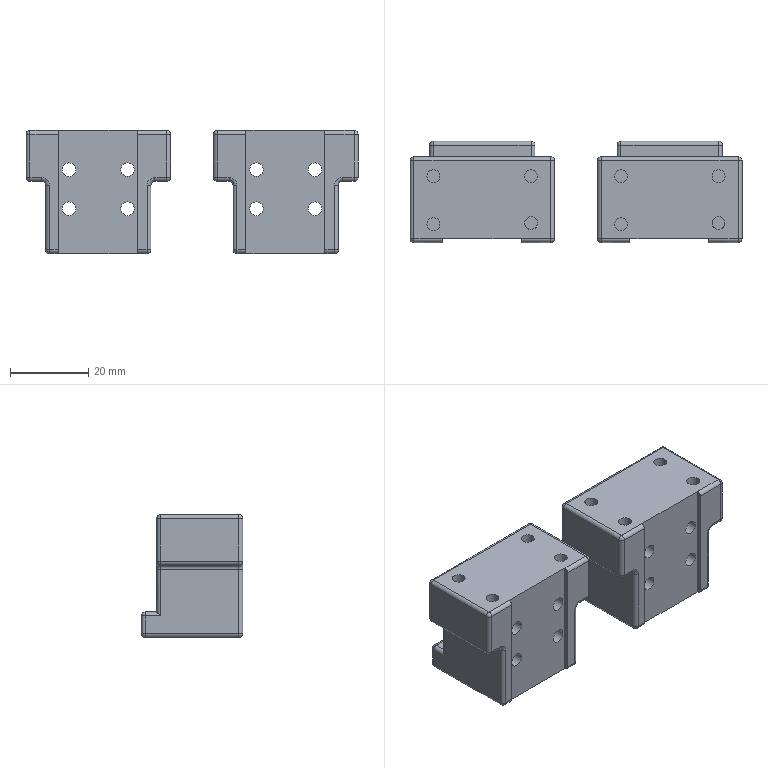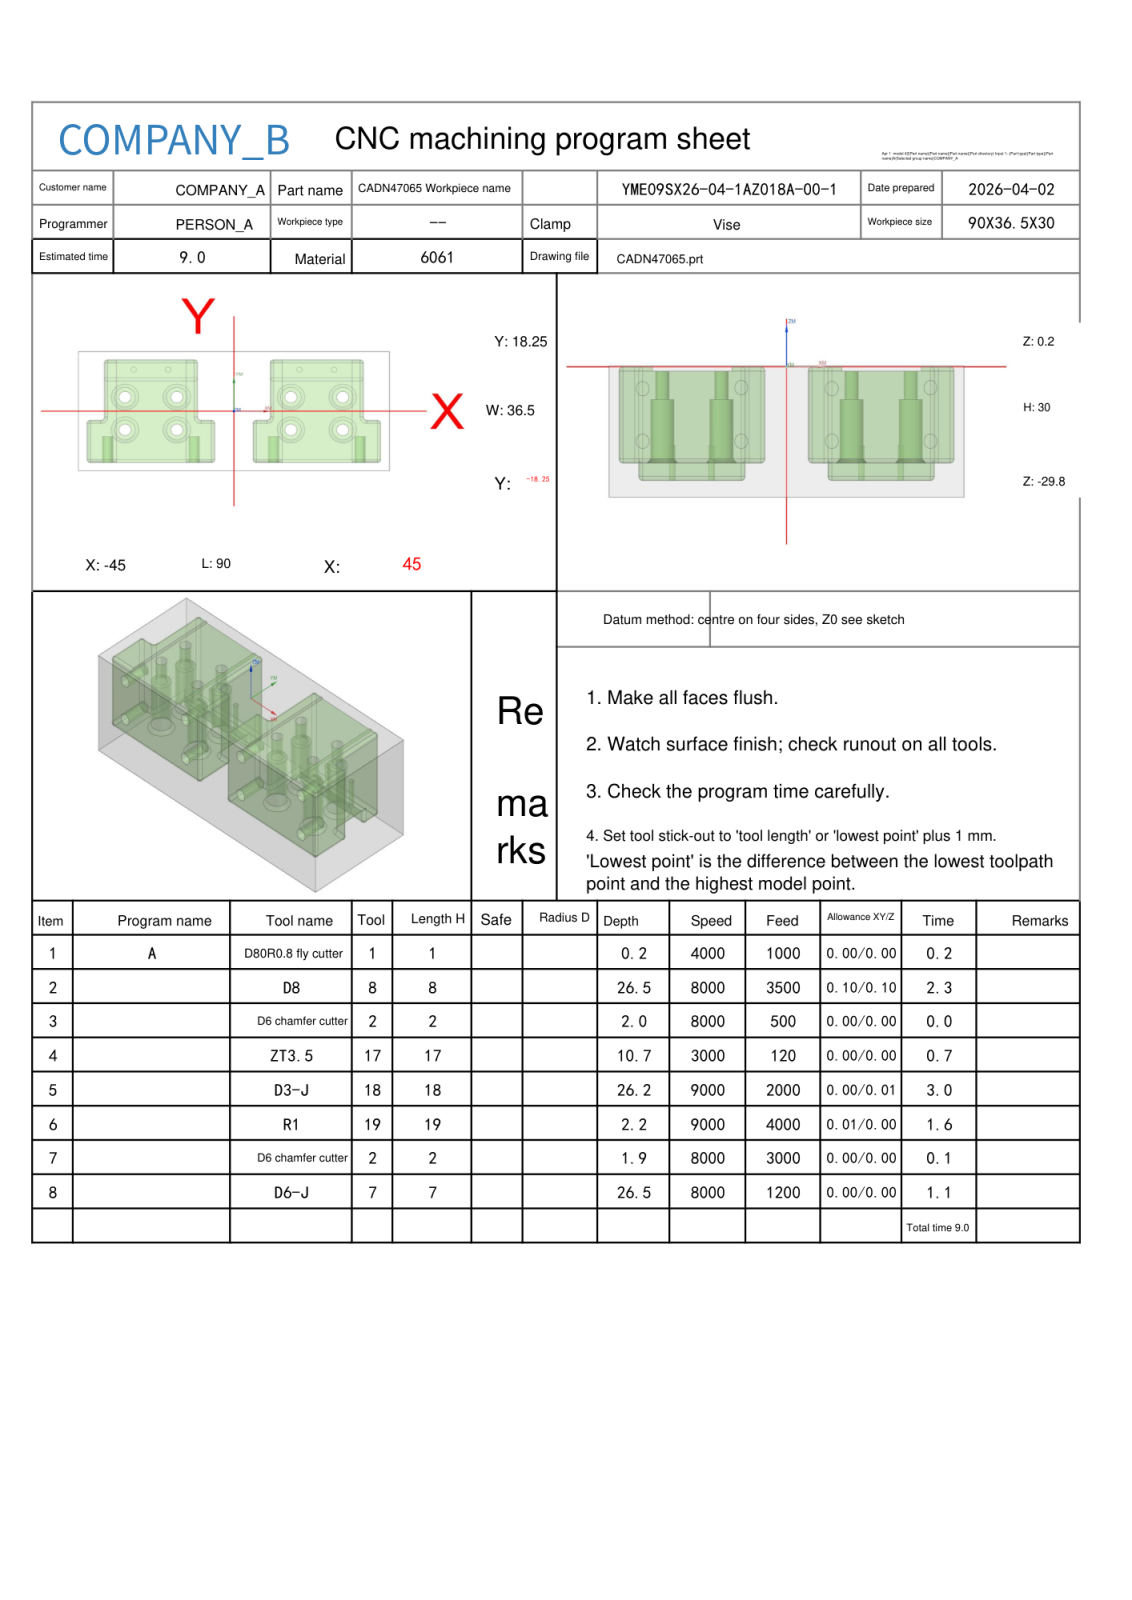NC program | NX | posted by the shop | part box 85 x 26 x 31.5 mm
Lines 3074 to 4231 of 17928:
N5 T18 M06
(D3-J  D=3. R=0. H=18 ce=0.00 di=0.01)
G00 G90 G54 X5.414 Y-.858 M03 S9000
G43 H18 Z20.
M08
Z-.75
G01 X5.417 Y-.864 Z-.818 F1600.
X5.424 Y-.88 Z-.88
X5.435 Y-.905 Z-.935
X5.45 Y-.937 Z-.983
X5.47 Y-.975 Z-1.026
X5.493 Y-1.017 Z-1.064
X5.519 Y-1.062 Z-1.095
X5.549 Y-1.108 Z-1.123
X5.582 Y-1.154 Z-1.145
X5.618 Y-1.198 Z-1.163
X5.656 Y-1.24 Z-1.177
X5.697 Y-1.276 Z-1.187
X5.739 Y-1.306 Z-1.194
X5.784 Y-1.328 Z-1.198
X5.831 Y-1.341 Z-1.2
G02 X6.5 Y-1.25 I.669 J-2.409 F2000.
G01 X9.
Y2.291
X8.985 Y2.32
X8.943 Y2.324 Z-1.202
X8.876 Y2.306 Z-1.205
X8.787 Y2.268 Z-1.208
X8.68 Y2.211 Z-1.213
X8.558 Y2.137 Z-1.218
X8.344 Y1.994 Z-1.228
X8.103 Y1.816 Z-1.239
X7.815 Y1.584 Z-1.254
X7.399 Y1.201 Z-1.276
X7.008 Y.785 Z-1.299
X6.651 Y.343 Z-1.323
X6.335 Y-.117 Z-1.345
X6.152 Y-.428 Z-1.359
X6.016 Y-.686 Z-1.371
X5.91 Y-.911 Z-1.38
X5.858 Y-1.038 Z-1.386
X5.82 Y-1.148 Z-1.39
X5.797 Y-1.236 Z-1.394
X5.79 Y-1.3 Z-1.397
X5.801 Y-1.336 Z-1.399
X5.831 Y-1.341
G02 X6.5 Y-1.25 I.669 J-2.409
G01 X9.
Y2.291
X8.985 Y2.32 Z-1.4
X8.943 Y2.324 Z-1.402
X8.876 Y2.306 Z-1.404
X8.787 Y2.268 Z-1.408
X8.68 Y2.211 Z-1.413
X8.558 Y2.137 Z-1.418
X8.344 Y1.994 Z-1.428
X8.103 Y1.816 Z-1.439
X7.815 Y1.584 Z-1.453
X7.399 Y1.201 Z-1.476
X7.008 Y.785 Z-1.499
X6.651 Y.343 Z-1.522
X6.335 Y-.117 Z-1.545
X6.152 Y-.428 Z-1.559
X6.016 Y-.686 Z-1.57
X5.91 Y-.911 Z-1.58
X5.858 Y-1.038 Z-1.585
X5.82 Y-1.148 Z-1.59
X5.797 Y-1.236 Z-1.594
X5.79 Y-1.3 Z-1.596
X5.801 Y-1.336 Z-1.598
X5.831 Y-1.341 Z-1.599
G02 X6.5 Y-1.25 I.669 J-2.409
G01 X9.
Y2.291
X8.985 Y2.32
X8.943 Y2.324 Z-1.601
X8.876 Y2.306 Z-1.604
X8.787 Y2.268 Z-1.608
X8.68 Y2.211 Z-1.612
X8.558 Y2.137 Z-1.618
X8.344 Y1.994 Z-1.627
X8.103 Y1.816 Z-1.639
X7.815 Y1.584 Z-1.653
X7.399 Y1.201 Z-1.675
X7.008 Y.785 Z-1.699
X6.651 Y.343 Z-1.722
X6.335 Y-.117 Z-1.744
X6.152 Y-.428 Z-1.759
X6.016 Y-.686 Z-1.77
X5.91 Y-.911 Z-1.78
X5.858 Y-1.038 Z-1.785
X5.82 Y-1.148 Z-1.79
X5.797 Y-1.236 Z-1.793
X5.79 Y-1.3 Z-1.796
X5.801 Y-1.336 Z-1.798
X5.831 Y-1.341
G02 X6.5 Y-1.25 I.669 J-2.409
G01 X9.
Y2.291
X8.985 Y2.32 Z-1.799
X8.943 Y2.324 Z-1.801
X8.876 Y2.306 Z-1.804
X8.787 Y2.268 Z-1.807
X8.68 Y2.211 Z-1.812
X8.558 Y2.137 Z-1.817
X8.344 Y1.994 Z-1.827
X8.103 Y1.816 Z-1.838
X7.815 Y1.584 Z-1.852
X7.399 Y1.201 Z-1.875
X7.008 Y.785 Z-1.898
X6.651 Y.343 Z-1.921
X6.335 Y-.117 Z-1.944
X6.152 Y-.428 Z-1.958
X6.016 Y-.686 Z-1.969
X5.91 Y-.911 Z-1.979
X5.858 Y-1.038 Z-1.984
X5.82 Y-1.148 Z-1.989
X5.797 Y-1.236 Z-1.993
X5.79 Y-1.3 Z-1.996
X5.801 Y-1.336 Z-1.997
X5.831 Y-1.341 Z-1.998
G02 X6.5 Y-1.25 I.669 J-2.409
G01 X9.
Y2.291
X8.985 Y2.32 Z-1.999
X8.943 Y2.324 Z-2.
X8.876 Y2.306 Z-2.003
X8.787 Y2.268 Z-2.007
X8.68 Y2.211 Z-2.012
X8.558 Y2.137 Z-2.017
X8.344 Y1.994 Z-2.027
X8.103 Y1.816 Z-2.038
X7.815 Y1.584 Z-2.052
X7.399 Y1.201 Z-2.075
X7.008 Y.785 Z-2.098
X6.651 Y.343 Z-2.121
X6.335 Y-.117 Z-2.144
X6.152 Y-.428 Z-2.158
X6.016 Y-.686 Z-2.169
X5.91 Y-.911 Z-2.179
X5.858 Y-1.038 Z-2.184
X5.82 Y-1.148 Z-2.189
X5.797 Y-1.236 Z-2.192
X5.79 Y-1.3 Z-2.195
X5.801 Y-1.336 Z-2.197
X5.831 Y-1.341 Z-2.198
G02 X6.5 Y-1.25 I.669 J-2.409
G01 X9.
Y2.291
X8.985 Y2.32
X8.943 Y2.324 Z-2.2
X8.876 Y2.306 Z-2.203
X8.787 Y2.268 Z-2.207
X8.68 Y2.211 Z-2.211
X8.558 Y2.137 Z-2.216
X8.344 Y1.994 Z-2.226
X8.103 Y1.816 Z-2.237
X7.815 Y1.584 Z-2.252
X7.399 Y1.201 Z-2.274
X7.008 Y.785 Z-2.297
X6.651 Y.343 Z-2.321
X6.335 Y-.117 Z-2.343
X6.152 Y-.428 Z-2.357
X6.016 Y-.686 Z-2.369
X5.91 Y-.911 Z-2.378
X5.858 Y-1.038 Z-2.384
X5.82 Y-1.148 Z-2.388
X5.797 Y-1.236 Z-2.392
X5.79 Y-1.3 Z-2.395
X5.801 Y-1.336 Z-2.397
X5.831 Y-1.341
G02 X6.5 Y-1.25 I.669 J-2.409
G01 X9.
Y2.291
X8.985 Y2.32 Z-2.398
X8.943 Y2.324 Z-2.4
X8.876 Y2.306 Z-2.402
X8.787 Y2.268 Z-2.406
X8.68 Y2.211 Z-2.411
X8.558 Y2.137 Z-2.416
X8.344 Y1.994 Z-2.426
X8.103 Y1.816 Z-2.437
X7.815 Y1.584 Z-2.451
X7.399 Y1.201 Z-2.474
X7.008 Y.785 Z-2.497
X6.651 Y.343 Z-2.52
X6.335 Y-.117 Z-2.543
X6.152 Y-.428 Z-2.557
X6.016 Y-.686 Z-2.568
X5.91 Y-.911 Z-2.578
X5.858 Y-1.038 Z-2.583
X5.82 Y-1.148 Z-2.588
X5.797 Y-1.236 Z-2.592
X5.79 Y-1.3 Z-2.594
X5.801 Y-1.336 Z-2.596
X5.831 Y-1.341 Z-2.597
G02 X6.5 Y-1.25 I.669 J-2.409
G01 X9.
Y2.291
X8.985 Y2.32
X8.943 Y2.324 Z-2.599
X8.876 Y2.306 Z-2.602
X8.787 Y2.268 Z-2.606
X8.68 Y2.211 Z-2.61
X8.558 Y2.137 Z-2.616
X8.344 Y1.994 Z-2.625
X8.103 Y1.816 Z-2.637
X7.815 Y1.584 Z-2.651
X7.399 Y1.201 Z-2.673
X7.008 Y.785 Z-2.697
X6.651 Y.343 Z-2.72
X6.335 Y-.117 Z-2.742
X6.152 Y-.428 Z-2.757
X6.016 Y-.686 Z-2.768
X5.91 Y-.911 Z-2.778
X5.858 Y-1.038 Z-2.783
X5.82 Y-1.148 Z-2.788
X5.797 Y-1.236 Z-2.791
X5.79 Y-1.3 Z-2.794
X5.801 Y-1.336 Z-2.796
X5.831 Y-1.341
G02 X6.5 Y-1.25 I.669 J-2.409
G01 X9.
Y2.291
X8.985 Y2.32 Z-2.797
X8.943 Y2.324 Z-2.799
X8.876 Y2.306 Z-2.802
X8.787 Y2.268 Z-2.805
X8.68 Y2.211 Z-2.81
X8.558 Y2.137 Z-2.815
X8.344 Y1.994 Z-2.825
X8.103 Y1.816 Z-2.836
X7.815 Y1.584 Z-2.85
X7.399 Y1.201 Z-2.873
X7.008 Y.785 Z-2.896
X6.651 Y.343 Z-2.919
X6.335 Y-.117 Z-2.942
X6.152 Y-.428 Z-2.956
X6.016 Y-.686 Z-2.967
X5.91 Y-.911 Z-2.977
X5.858 Y-1.038 Z-2.982
X5.82 Y-1.148 Z-2.987
X5.797 Y-1.236 Z-2.991
X5.79 Y-1.3 Z-2.994
X5.801 Y-1.336 Z-2.995
X5.831 Y-1.341 Z-2.996
G02 X6.5 Y-1.25 I.669 J-2.409
G01 X9.
Y2.291
X8.985 Y2.32 Z-2.997
X8.943 Y2.324 Z-2.998
X8.876 Y2.306 Z-3.001
X8.787 Y2.268 Z-3.005
X8.68 Y2.211 Z-3.01
X8.558 Y2.137 Z-3.015
X8.344 Y1.994 Z-3.025
X8.103 Y1.816 Z-3.036
X7.815 Y1.584 Z-3.05
X7.399 Y1.201 Z-3.073
X7.008 Y.785 Z-3.096
X6.651 Y.343 Z-3.119
X6.335 Y-.117 Z-3.142
X6.152 Y-.428 Z-3.156
X6.016 Y-.686 Z-3.167
X5.91 Y-.911 Z-3.177
X5.858 Y-1.038 Z-3.182
X5.82 Y-1.148 Z-3.187
X5.797 Y-1.236 Z-3.19
X5.79 Y-1.3 Z-3.193
X5.801 Y-1.336 Z-3.195
X5.831 Y-1.341 Z-3.196
G02 X6.5 Y-1.25 I.669 J-2.409
G01 X9.
Y2.291
X8.985 Y2.32
X8.943 Y2.324 Z-3.198
X8.876 Y2.306 Z-3.201
X8.787 Y2.268 Z-3.205
X8.68 Y2.211 Z-3.209
X8.558 Y2.137 Z-3.215
X8.344 Y1.994 Z-3.224
X8.103 Y1.816 Z-3.235
X7.815 Y1.584 Z-3.25
X7.399 Y1.201 Z-3.272
X7.008 Y.785 Z-3.295
X6.651 Y.343 Z-3.319
X6.335 Y-.117 Z-3.341
X6.152 Y-.428 Z-3.355
X6.016 Y-.686 Z-3.367
X5.91 Y-.911 Z-3.376
X5.858 Y-1.038 Z-3.382
X5.82 Y-1.148 Z-3.386
X5.797 Y-1.236 Z-3.39
X5.79 Y-1.3 Z-3.393
X5.801 Y-1.336 Z-3.395
X5.831 Y-1.341
G02 X6.5 Y-1.25 I.669 J-2.409
G01 X9.
Y2.291
X8.985 Y2.32 Z-3.396
X8.943 Y2.324 Z-3.398
X8.876 Y2.306 Z-3.4
X8.787 Y2.268 Z-3.404
X8.68 Y2.211 Z-3.409
X8.558 Y2.137 Z-3.414
X8.344 Y1.994 Z-3.424
X8.103 Y1.816 Z-3.435
X7.815 Y1.584 Z-3.449
X7.399 Y1.201 Z-3.472
X7.008 Y.785 Z-3.495
X6.651 Y.343 Z-3.518
X6.335 Y-.117 Z-3.541
X6.152 Y-.428 Z-3.555
X6.016 Y-.686 Z-3.566
X5.91 Y-.911 Z-3.576
X5.858 Y-1.038 Z-3.581
X5.82 Y-1.148 Z-3.586
X5.797 Y-1.236 Z-3.59
X5.79 Y-1.3 Z-3.592
X5.801 Y-1.336 Z-3.594
X5.831 Y-1.341 Z-3.595
G02 X6.5 Y-1.25 I.669 J-2.409
G01 X9.
Y2.291
X8.985 Y2.32
X8.943 Y2.324 Z-3.597
X8.876 Y2.306 Z-3.6
X8.787 Y2.268 Z-3.604
X8.68 Y2.211 Z-3.608
X8.558 Y2.137 Z-3.614
X8.344 Y1.994 Z-3.623
X8.103 Y1.816 Z-3.635
X7.815 Y1.584 Z-3.649
X7.399 Y1.201 Z-3.671
X7.008 Y.785 Z-3.695
X6.651 Y.343 Z-3.718
X6.335 Y-.117 Z-3.74
X6.152 Y-.428 Z-3.755
X6.016 Y-.686 Z-3.766
X5.91 Y-.911 Z-3.776
X5.858 Y-1.038 Z-3.781
X5.82 Y-1.148 Z-3.786
X5.797 Y-1.236 Z-3.789
X5.79 Y-1.3 Z-3.792
X5.801 Y-1.336 Z-3.794
X5.831 Y-1.341
G02 X6.5 Y-1.25 I.669 J-2.409
G01 X9.
Y2.291
X8.985 Y2.32 Z-3.795
X8.943 Y2.324 Z-3.797
X8.876 Y2.306 Z-3.8
X8.787 Y2.268 Z-3.803
X8.68 Y2.211 Z-3.808
X8.558 Y2.137 Z-3.813
X8.344 Y1.994 Z-3.823
X8.103 Y1.816 Z-3.834
X7.815 Y1.584 Z-3.848
X7.399 Y1.201 Z-3.871
X7.008 Y.785 Z-3.894
X6.651 Y.343 Z-3.917
X6.335 Y-.117 Z-3.94
X6.152 Y-.428 Z-3.954
X6.016 Y-.686 Z-3.965
X5.91 Y-.911 Z-3.975
X5.858 Y-1.038 Z-3.98
X5.82 Y-1.148 Z-3.985
X5.797 Y-1.236 Z-3.989
X5.79 Y-1.3 Z-3.992
X5.801 Y-1.336 Z-3.993
X5.831 Y-1.341 Z-3.994
G02 X6.5 Y-1.25 I.669 J-2.409
G01 X9.
Y2.291
X8.985 Y2.32 Z-3.995
X8.943 Y2.324 Z-3.996
X8.876 Y2.306 Z-3.999
X8.787 Y2.268 Z-4.003
X8.68 Y2.211 Z-4.008
X8.558 Y2.137 Z-4.013
X8.344 Y1.994 Z-4.023
X8.103 Y1.816 Z-4.034
X7.815 Y1.584 Z-4.048
X7.399 Y1.201 Z-4.071
X7.008 Y.785 Z-4.094
X6.651 Y.343 Z-4.117
X6.335 Y-.117 Z-4.14
X6.152 Y-.428 Z-4.154
X6.016 Y-.686 Z-4.165
X5.91 Y-.911 Z-4.175
X5.858 Y-1.038 Z-4.18
X5.82 Y-1.148 Z-4.185
X5.797 Y-1.236 Z-4.188
X5.79 Y-1.3 Z-4.191
X5.801 Y-1.336 Z-4.193
X5.831 Y-1.341 Z-4.194
G02 X6.5 Y-1.25 I.669 J-2.409
G01 X9.
Y2.291
X8.985 Y2.32
X8.943 Y2.324 Z-4.196
X8.876 Y2.306 Z-4.199
X8.787 Y2.268 Z-4.203
X8.68 Y2.211 Z-4.207
X8.558 Y2.137 Z-4.213
X8.344 Y1.994 Z-4.222
X8.103 Y1.816 Z-4.233
X7.815 Y1.584 Z-4.248
X7.399 Y1.201 Z-4.27
X7.008 Y.785 Z-4.293
X6.651 Y.343 Z-4.317
X6.335 Y-.117 Z-4.339
X6.152 Y-.428 Z-4.353
X6.016 Y-.686 Z-4.365
X5.91 Y-.911 Z-4.374
X5.858 Y-1.038 Z-4.38
X5.82 Y-1.148 Z-4.384
X5.797 Y-1.236 Z-4.388
X5.79 Y-1.3 Z-4.391
X5.801 Y-1.336 Z-4.393
X5.831 Y-1.341
G02 X6.5 Y-1.25 I.669 J-2.409
G01 X9.
Y2.291
X8.985 Y2.32 Z-4.394
X8.943 Y2.324 Z-4.396
X8.876 Y2.306 Z-4.398
X8.787 Y2.268 Z-4.402
X8.68 Y2.211 Z-4.407
X8.558 Y2.137 Z-4.412
X8.344 Y1.994 Z-4.422
X8.103 Y1.816 Z-4.433
X7.815 Y1.584 Z-4.447
X7.399 Y1.201 Z-4.47
X7.008 Y.785 Z-4.493
X6.651 Y.343 Z-4.516
X6.335 Y-.117 Z-4.539
X6.152 Y-.428 Z-4.553
X6.016 Y-.686 Z-4.564
X5.91 Y-.911 Z-4.574
X5.858 Y-1.038 Z-4.579
X5.82 Y-1.148 Z-4.584
X5.797 Y-1.236 Z-4.588
X5.79 Y-1.3 Z-4.59
X5.801 Y-1.336 Z-4.592
X5.831 Y-1.341 Z-4.593
G02 X6.5 Y-1.25 I.669 J-2.409
G01 X9.
Y2.291
X8.985 Y2.32
X8.943 Y2.324 Z-4.595
X8.876 Y2.306 Z-4.598
X8.787 Y2.268 Z-4.602
X8.68 Y2.211 Z-4.606
X8.558 Y2.137 Z-4.612
X8.344 Y1.994 Z-4.621
X8.103 Y1.816 Z-4.633
X7.815 Y1.584 Z-4.647
X7.399 Y1.201 Z-4.669
X7.008 Y.785 Z-4.693
X6.651 Y.343 Z-4.716
X6.335 Y-.117 Z-4.738
X6.152 Y-.428 Z-4.753
X6.016 Y-.686 Z-4.764
X5.91 Y-.911 Z-4.774
X5.858 Y-1.038 Z-4.779
X5.82 Y-1.148 Z-4.784
X5.797 Y-1.236 Z-4.787
X5.79 Y-1.3 Z-4.79
X5.801 Y-1.336 Z-4.792
X5.831 Y-1.341
G02 X6.5 Y-1.25 I.669 J-2.409
G01 X9.
Y2.291
X8.985 Y2.32 Z-4.793
X8.943 Y2.324 Z-4.795
X8.876 Y2.306 Z-4.798
X8.787 Y2.268 Z-4.801
X8.68 Y2.211 Z-4.806
X8.558 Y2.137 Z-4.811
X8.344 Y1.994 Z-4.821
X8.103 Y1.816 Z-4.832
X7.815 Y1.584 Z-4.846
X7.399 Y1.201 Z-4.869
X7.008 Y.785 Z-4.892
X6.651 Y.343 Z-4.915
X6.335 Y-.117 Z-4.938
X6.152 Y-.428 Z-4.952
X6.016 Y-.686 Z-4.963
X5.91 Y-.911 Z-4.973
X5.858 Y-1.038 Z-4.978
X5.82 Y-1.148 Z-4.983
X5.797 Y-1.236 Z-4.987
X5.79 Y-1.3 Z-4.99
X5.801 Y-1.336 Z-4.991
X5.831 Y-1.341 Z-4.992
G02 X6.5 Y-1.25 I.669 J-2.409
G01 X9.
Y2.291
X8.985 Y2.32 Z-4.993
X8.943 Y2.324 Z-4.994
X8.876 Y2.306 Z-4.997
X8.787 Y2.268 Z-5.001
X8.68 Y2.211 Z-5.006
X8.558 Y2.137 Z-5.011
X8.344 Y1.994 Z-5.021
X8.103 Y1.816 Z-5.032
X7.815 Y1.584 Z-5.046
X7.399 Y1.201 Z-5.069
X7.008 Y.785 Z-5.092
X6.651 Y.343 Z-5.115
X6.335 Y-.117 Z-5.138
X6.152 Y-.428 Z-5.152
X6.016 Y-.686 Z-5.163
X5.91 Y-.911 Z-5.173
X5.858 Y-1.038 Z-5.178
X5.82 Y-1.148 Z-5.183
X5.797 Y-1.236 Z-5.186
X5.79 Y-1.3 Z-5.189
X5.801 Y-1.336 Z-5.191
X5.831 Y-1.341 Z-5.192
G02 X6.5 Y-1.25 I.669 J-2.409
G01 X9.
Y2.291
X8.985 Y2.32
X8.943 Y2.324 Z-5.194
X8.876 Y2.306 Z-5.197
X8.787 Y2.268 Z-5.201
X8.68 Y2.211 Z-5.205
X8.558 Y2.137 Z-5.211
X8.344 Y1.994 Z-5.22
X8.103 Y1.816 Z-5.231
X7.815 Y1.584 Z-5.246
X7.399 Y1.201 Z-5.268
X7.008 Y.785 Z-5.291
X6.651 Y.343 Z-5.315
X6.335 Y-.117 Z-5.337
X6.152 Y-.428 Z-5.351
X6.016 Y-.686 Z-5.363
X5.91 Y-.911 Z-5.372
X5.858 Y-1.038 Z-5.378
X5.82 Y-1.148 Z-5.382
X5.797 Y-1.236 Z-5.386
X5.79 Y-1.3 Z-5.389
X5.801 Y-1.336 Z-5.391
X5.831 Y-1.341
G02 X6.5 Y-1.25 I.669 J-2.409
G01 X9.
Y2.291
X8.985 Y2.32 Z-5.392
X8.943 Y2.324 Z-5.394
X8.876 Y2.306 Z-5.396
X8.787 Y2.268 Z-5.4
X8.68 Y2.211 Z-5.405
X8.558 Y2.137 Z-5.41
X8.344 Y1.994 Z-5.42
X8.103 Y1.816 Z-5.431
X7.815 Y1.584 Z-5.445
X7.399 Y1.201 Z-5.468
X7.008 Y.785 Z-5.491
X6.651 Y.343 Z-5.514
X6.335 Y-.117 Z-5.537
X6.152 Y-.428 Z-5.551
X6.016 Y-.686 Z-5.562
X5.91 Y-.911 Z-5.572
X5.858 Y-1.038 Z-5.577
X5.82 Y-1.148 Z-5.582
X5.797 Y-1.236 Z-5.586
X5.79 Y-1.3 Z-5.588
X5.801 Y-1.336 Z-5.59
X5.831 Y-1.341 Z-5.591
G02 X6.5 Y-1.25 I.669 J-2.409
G01 X9.
Y2.291
X8.985 Y2.32
X8.943 Y2.324 Z-5.593
X8.876 Y2.306 Z-5.596
X8.787 Y2.268 Z-5.6
X8.68 Y2.211 Z-5.604
X8.558 Y2.137 Z-5.61
X8.344 Y1.994 Z-5.619
X8.103 Y1.816 Z-5.631
X7.815 Y1.584 Z-5.645
X7.399 Y1.201 Z-5.667
X7.008 Y.785 Z-5.691
X6.651 Y.343 Z-5.714
X6.335 Y-.117 Z-5.736
X6.152 Y-.428 Z-5.751
X6.016 Y-.686 Z-5.762
X5.91 Y-.911 Z-5.772
X5.858 Y-1.038 Z-5.777
X5.82 Y-1.148 Z-5.782
X5.797 Y-1.236 Z-5.785
X5.79 Y-1.3 Z-5.788
X5.801 Y-1.336 Z-5.79
X5.831 Y-1.341
G02 X6.5 Y-1.25 I.669 J-2.409
G01 X9.
Y2.291
X8.985 Y2.32 Z-5.791
X8.943 Y2.324 Z-5.793
X8.876 Y2.306 Z-5.796
X8.787 Y2.268 Z-5.799
X8.68 Y2.211 Z-5.804
X8.558 Y2.137 Z-5.809
X8.344 Y1.994 Z-5.819
X8.103 Y1.816 Z-5.83
X7.815 Y1.584 Z-5.844
X7.399 Y1.201 Z-5.867
X7.008 Y.785 Z-5.89
X6.651 Y.343 Z-5.913
X6.335 Y-.117 Z-5.936
X6.152 Y-.428 Z-5.95
X6.016 Y-.686 Z-5.961
X5.91 Y-.911 Z-5.971
X5.858 Y-1.038 Z-5.976
X5.82 Y-1.148 Z-5.981
X5.797 Y-1.236 Z-5.985
X5.79 Y-1.3 Z-5.988
X5.801 Y-1.336 Z-5.989
X5.831 Y-1.341 Z-5.99
G02 X6.5 Y-1.25 I.669 J-2.409
G01 X9.
Y2.291
X8.985 Y2.32 Z-5.991
X8.943 Y2.324 Z-5.992
X8.876 Y2.306 Z-5.995
X8.787 Y2.268 Z-5.999
X8.68 Y2.211 Z-6.004
X8.558 Y2.137 Z-6.009
X8.344 Y1.994 Z-6.019
X8.103 Y1.816 Z-6.03
X7.815 Y1.584 Z-6.044
X7.399 Y1.201 Z-6.067
X7.008 Y.785 Z-6.09
X6.651 Y.343 Z-6.113
X6.335 Y-.117 Z-6.136
X6.152 Y-.428 Z-6.15
X6.016 Y-.686 Z-6.161
X5.91 Y-.911 Z-6.171
X5.858 Y-1.038 Z-6.176
X5.82 Y-1.148 Z-6.181
X5.797 Y-1.236 Z-6.184
X5.79 Y-1.3 Z-6.187
X5.801 Y-1.336 Z-6.189
X5.831 Y-1.341 Z-6.19
G02 X6.5 Y-1.25 I.669 J-2.409
G01 X9.
Y2.291
X8.985 Y2.32
X8.943 Y2.324 Z-6.192
X8.876 Y2.306 Z-6.195
X8.787 Y2.268 Z-6.199
X8.68 Y2.211 Z-6.203
X8.558 Y2.137 Z-6.209
X8.344 Y1.994 Z-6.218
X8.103 Y1.816 Z-6.229
X7.815 Y1.584 Z-6.244
X7.399 Y1.201 Z-6.266
X7.008 Y.785 Z-6.289
X6.651 Y.343 Z-6.313
X6.335 Y-.117 Z-6.335
X6.152 Y-.428 Z-6.349
X6.016 Y-.686 Z-6.361
X5.91 Y-.911 Z-6.37
X5.858 Y-1.038 Z-6.376
X5.82 Y-1.148 Z-6.38
X5.797 Y-1.236 Z-6.384
X5.79 Y-1.3 Z-6.387
X5.801 Y-1.336 Z-6.389
X5.831 Y-1.341
G02 X6.5 Y-1.25 I.669 J-2.409
G01 X9.
Y2.291
X8.985 Y2.32 Z-6.39
X8.943 Y2.324 Z-6.392
X8.876 Y2.306 Z-6.394
X8.787 Y2.268 Z-6.398
X8.68 Y2.211 Z-6.403
X8.558 Y2.137 Z-6.408
X8.344 Y1.994 Z-6.418
X8.103 Y1.816 Z-6.429
X7.815 Y1.584 Z-6.443
X7.399 Y1.201 Z-6.466
X7.008 Y.785 Z-6.489
X6.651 Y.343 Z-6.512
X6.335 Y-.117 Z-6.535
X6.152 Y-.428 Z-6.549
X6.016 Y-.686 Z-6.56
X5.91 Y-.911 Z-6.57
X5.858 Y-1.038 Z-6.575
X5.82 Y-1.148 Z-6.58
X5.797 Y-1.236 Z-6.584
X5.79 Y-1.3 Z-6.586
X5.801 Y-1.336 Z-6.588
X5.831 Y-1.341 Z-6.589
G02 X6.5 Y-1.25 I.669 J-2.409
G01 X9.
Y2.291
X8.985 Y2.32
X8.943 Y2.324 Z-6.591
X8.876 Y2.306 Z-6.594
X8.787 Y2.268 Z-6.598
X8.68 Y2.211 Z-6.602
X8.558 Y2.137 Z-6.608
X8.344 Y1.994 Z-6.617
X8.103 Y1.816 Z-6.629
X7.815 Y1.584 Z-6.643
X7.399 Y1.201 Z-6.665
X7.008 Y.785 Z-6.689
X6.651 Y.343 Z-6.712
X6.335 Y-.117 Z-6.734
X6.152 Y-.428 Z-6.749
X6.016 Y-.686 Z-6.76
X5.91 Y-.911 Z-6.77
X5.858 Y-1.038 Z-6.775
X5.82 Y-1.148 Z-6.78
X5.797 Y-1.236 Z-6.783
X5.79 Y-1.3 Z-6.786
X5.801 Y-1.336 Z-6.788
X5.831 Y-1.341
G02 X6.5 Y-1.25 I.669 J-2.409
G01 X9.
Y2.291
X8.985 Y2.32 Z-6.789
X8.943 Y2.324 Z-6.791
X8.876 Y2.306 Z-6.794
X8.787 Y2.268 Z-6.797
X8.68 Y2.211 Z-6.802
X8.558 Y2.137 Z-6.807
X8.344 Y1.994 Z-6.817
X8.103 Y1.816 Z-6.828
X7.815 Y1.584 Z-6.842
X7.399 Y1.201 Z-6.865
X7.008 Y.785 Z-6.888
X6.651 Y.343 Z-6.911
X6.335 Y-.117 Z-6.934
X6.152 Y-.428 Z-6.948
X6.016 Y-.686 Z-6.959
X5.91 Y-.911 Z-6.969
X5.858 Y-1.038 Z-6.975
X5.82 Y-1.148 Z-6.979
X5.797 Y-1.236 Z-6.983
X5.79 Y-1.3 Z-6.986
X5.801 Y-1.336 Z-6.987
X5.831 Y-1.341 Z-6.988
G02 X6.5 Y-1.25 I.669 J-2.409
G01 X9.
Y2.291
X8.985 Y2.32 Z-6.989
X8.943 Y2.324 Z-6.99
X8.876 Y2.306 Z-6.993
X8.787 Y2.268 Z-6.997
X8.68 Y2.211 Z-7.002
X8.558 Y2.137 Z-7.007
X8.344 Y1.994 Z-7.017
X8.103 Y1.816 Z-7.028
X7.815 Y1.584 Z-7.042
X7.399 Y1.201 Z-7.065
X7.008 Y.785 Z-7.088
X6.651 Y.343 Z-7.111
X6.335 Y-.117 Z-7.134
X6.152 Y-.428 Z-7.148
X6.016 Y-.686 Z-7.159
X5.91 Y-.911 Z-7.169
X5.858 Y-1.038 Z-7.174
X5.82 Y-1.148 Z-7.179
X5.797 Y-1.236 Z-7.182
X5.79 Y-1.3 Z-7.185
X5.801 Y-1.336 Z-7.187
X5.831 Y-1.341 Z-7.188
G02 X6.5 Y-1.25 I.669 J-2.409
G01 X9.
Y2.291
X8.985 Y2.32
X8.943 Y2.324 Z-7.19
X8.876 Y2.306 Z-7.193
X8.787 Y2.268 Z-7.197
X8.68 Y2.211 Z-7.201
X8.558 Y2.137 Z-7.207
X8.344 Y1.994 Z-7.216
X8.103 Y1.816 Z-7.227
X7.815 Y1.584 Z-7.242
X7.399 Y1.201 Z-7.264
X7.008 Y.785 Z-7.287
X6.651 Y.343 Z-7.311
X6.335 Y-.117 Z-7.333
X6.152 Y-.428 Z-7.347
X6.016 Y-.686 Z-7.359
X5.91 Y-.911 Z-7.368
X5.858 Y-1.038 Z-7.374
X5.82 Y-1.148 Z-7.378
X5.797 Y-1.236 Z-7.382
X5.79 Y-1.3 Z-7.385
X5.801 Y-1.336 Z-7.387
X5.831 Y-1.341
G02 X6.5 Y-1.25 I.669 J-2.409
G01 X9.
Y2.291
X8.985 Y2.32 Z-7.388
X8.943 Y2.324 Z-7.39
X8.876 Y2.306 Z-7.392
X8.787 Y2.268 Z-7.396
X8.68 Y2.211 Z-7.401
X8.558 Y2.137 Z-7.406
X8.344 Y1.994 Z-7.416
X8.103 Y1.816 Z-7.427
X7.815 Y1.584 Z-7.441
X7.399 Y1.201 Z-7.464
X7.008 Y.785 Z-7.487
X6.651 Y.343 Z-7.51
X6.335 Y-.117 Z-7.533
X6.152 Y-.428 Z-7.547
X6.016 Y-.686 Z-7.558
X5.91 Y-.911 Z-7.568
X5.858 Y-1.038 Z-7.573
X5.82 Y-1.148 Z-7.578
X5.797 Y-1.236 Z-7.582
X5.79 Y-1.3 Z-7.584
X5.801 Y-1.336 Z-7.586
X5.831 Y-1.341 Z-7.587
G02 X6.5 Y-1.25 I.669 J-2.409
G01 X9.
Y2.291
X8.985 Y2.32
X8.943 Y2.324 Z-7.589
X8.876 Y2.306 Z-7.592
X8.787 Y2.268 Z-7.596
X8.68 Y2.211 Z-7.6
X8.558 Y2.137 Z-7.606
X8.344 Y1.994 Z-7.615
X8.103 Y1.816 Z-7.627
X7.815 Y1.584 Z-7.641
X7.399 Y1.201 Z-7.663
X7.008 Y.785 Z-7.687
X6.651 Y.343 Z-7.71
X6.335 Y-.117 Z-7.732
X6.152 Y-.428 Z-7.747
X6.016 Y-.686 Z-7.758
X5.91 Y-.911 Z-7.768
X5.858 Y-1.038 Z-7.773
X5.82 Y-1.148 Z-7.778
X5.797 Y-1.236 Z-7.781
X5.79 Y-1.3 Z-7.784
X5.801 Y-1.336 Z-7.786
X5.831 Y-1.341
G02 X6.5 Y-1.25 I.669 J-2.409
G01 X9.
Y2.291
X8.985 Y2.32 Z-7.787
X8.943 Y2.324 Z-7.789
X8.876 Y2.306 Z-7.792
X8.787 Y2.268 Z-7.795
X8.68 Y2.211 Z-7.8
X8.558 Y2.137 Z-7.805
X8.344 Y1.994 Z-7.815
X8.103 Y1.816 Z-7.826
X7.815 Y1.584 Z-7.84
X7.399 Y1.201 Z-7.863
X7.008 Y.785 Z-7.886
X6.651 Y.343 Z-7.909
X6.335 Y-.117 Z-7.932
X6.152 Y-.428 Z-7.946
X6.016 Y-.686 Z-7.957
X5.91 Y-.911 Z-7.967
X5.858 Y-1.038 Z-7.973
X5.82 Y-1.148 Z-7.977
X5.797 Y-1.236 Z-7.981
X5.79 Y-1.3 Z-7.984
X5.801 Y-1.336 Z-7.985
X5.831 Y-1.341 Z-7.986
G02 X6.5 Y-1.25 I.669 J-2.409
G01 X9.
Y2.291
X8.985 Y2.32 Z-7.987
X8.943 Y2.324 Z-7.988
X8.876 Y2.306 Z-7.991
X8.787 Y2.268 Z-7.995
X8.68 Y2.211 Z-8.
X8.558 Y2.137 Z-8.005
X8.344 Y1.994 Z-8.015
X8.103 Y1.816 Z-8.026
X7.815 Y1.584 Z-8.04
X7.399 Y1.201 Z-8.063
X7.008 Y.785 Z-8.086
X6.651 Y.343 Z-8.109
X6.335 Y-.117 Z-8.132
X6.152 Y-.428 Z-8.146
X6.016 Y-.686 Z-8.157
X5.91 Y-.911 Z-8.167
X5.858 Y-1.038 Z-8.172
X5.82 Y-1.148 Z-8.177
X5.797 Y-1.236 Z-8.18
X5.79 Y-1.3 Z-8.183
X5.801 Y-1.336 Z-8.185
X5.831 Y-1.341 Z-8.186
G02 X6.5 Y-1.25 I.669 J-2.409
G01 X9.
Y2.291
X8.985 Y2.32
X8.943 Y2.324 Z-8.188
X8.876 Y2.306 Z-8.191
X8.787 Y2.268 Z-8.195
X8.68 Y2.211 Z-8.199
X8.558 Y2.137 Z-8.205
X8.344 Y1.994 Z-8.214
X8.103 Y1.816 Z-8.225
X7.815 Y1.584 Z-8.24
X7.399 Y1.201 Z-8.262
X7.008 Y.785 Z-8.285
X6.651 Y.343 Z-8.309
X6.335 Y-.117 Z-8.331
X6.152 Y-.428 Z-8.345
X6.016 Y-.686 Z-8.357
X5.91 Y-.911 Z-8.366
X5.858 Y-1.038 Z-8.372
X5.82 Y-1.148 Z-8.376
X5.797 Y-1.236 Z-8.38
X5.79 Y-1.3 Z-8.383
X5.801 Y-1.336 Z-8.385
X5.831 Y-1.341
G02 X6.5 Y-1.25 I.669 J-2.409
G01 X9.
Y2.291
X8.985 Y2.32 Z-8.386
X8.943 Y2.324 Z-8.388
X8.876 Y2.306 Z-8.39
X8.787 Y2.268 Z-8.394
X8.68 Y2.211 Z-8.399
X8.558 Y2.137 Z-8.404
X8.344 Y1.994 Z-8.414
X8.103 Y1.816 Z-8.425
X7.815 Y1.584 Z-8.439
X7.399 Y1.201 Z-8.462
X7.008 Y.785 Z-8.485
X6.651 Y.343 Z-8.508
X6.335 Y-.117 Z-8.531
X6.152 Y-.428 Z-8.545
X6.016 Y-.686 Z-8.556
X5.91 Y-.911 Z-8.566
X5.858 Y-1.038 Z-8.571
X5.82 Y-1.148 Z-8.576
X5.797 Y-1.236 Z-8.58
X5.79 Y-1.3 Z-8.582
X5.801 Y-1.336 Z-8.584
X5.831 Y-1.341 Z-8.585
G02 X6.5 Y-1.25 I.669 J-2.409
G01 X9.
Y2.291
X8.985 Y2.32
X8.943 Y2.324 Z-8.587
X8.876 Y2.306 Z-8.59
X8.787 Y2.268 Z-8.594
X8.68 Y2.211 Z-8.598
X8.558 Y2.137 Z-8.604
X8.344 Y1.994 Z-8.613
X8.103 Y1.816 Z-8.625
X7.815 Y1.584 Z-8.639
X7.399 Y1.201 Z-8.661
X7.008 Y.785 Z-8.685
X6.651 Y.343 Z-8.708
X6.335 Y-.117 Z-8.73
X6.152 Y-.428 Z-8.745
X6.016 Y-.686 Z-8.756
X5.91 Y-.911 Z-8.766
X5.858 Y-1.038 Z-8.771
X5.82 Y-1.148 Z-8.776
X5.797 Y-1.236 Z-8.779
X5.79 Y-1.3 Z-8.782
X5.801 Y-1.336 Z-8.784
X5.831 Y-1.341
G02 X6.5 Y-1.25 I.669 J-2.409
G01 X9.
Y2.291
X8.985 Y2.32 Z-8.785
X8.943 Y2.324 Z-8.787
X8.876 Y2.306 Z-8.79
X8.787 Y2.268 Z-8.793
X8.68 Y2.211 Z-8.798
X8.558 Y2.137 Z-8.803
X8.344 Y1.994 Z-8.813
X8.103 Y1.816 Z-8.824
X7.815 Y1.584 Z-8.838
X7.399 Y1.201 Z-8.861
X7.008 Y.785 Z-8.884
X6.651 Y.343 Z-8.907
X6.335 Y-.117 Z-8.93
X6.152 Y-.428 Z-8.944
X6.016 Y-.686 Z-8.955
X5.91 Y-.911 Z-8.965
X5.858 Y-1.038 Z-8.971
X5.82 Y-1.148 Z-8.975
X5.797 Y-1.236 Z-8.979
X5.79 Y-1.3 Z-8.982
X5.801 Y-1.336 Z-8.983
X5.831 Y-1.341 Z-8.984
G02 X6.5 Y-1.25 I.669 J-2.409
G01 X9.
Y2.291
X8.985 Y2.32 Z-8.985
X8.943 Y2.324 Z-8.986
X8.876 Y2.306 Z-8.989
X8.787 Y2.268 Z-8.993
X8.68 Y2.211 Z-8.998
X8.558 Y2.137 Z-9.003
X8.344 Y1.994 Z-9.013
X8.103 Y1.816 Z-9.024
X7.815 Y1.584 Z-9.038
X7.399 Y1.201 Z-9.061
X7.008 Y.785 Z-9.084
X6.651 Y.343 Z-9.107
X6.335 Y-.117 Z-9.13
X6.152 Y-.428 Z-9.144
X6.016 Y-.686 Z-9.155
X5.91 Y-.911 Z-9.165
X5.858 Y-1.038 Z-9.17
X5.82 Y-1.148 Z-9.175
X5.797 Y-1.236 Z-9.178
X5.79 Y-1.3 Z-9.181
X5.801 Y-1.336 Z-9.183
X5.831 Y-1.341 Z-9.184
G02 X6.5 Y-1.25 I.669 J-2.409
G01 X9.
Y2.291
X8.985 Y2.32
X8.943 Y2.324 Z-9.186
X8.876 Y2.306 Z-9.189
X8.787 Y2.268 Z-9.193
X8.68 Y2.211 Z-9.197
X8.558 Y2.137 Z-9.203
X8.344 Y1.994 Z-9.212
X8.103 Y1.816 Z-9.223
X7.815 Y1.584 Z-9.238
X7.399 Y1.201 Z-9.26
X7.008 Y.785 Z-9.283
X6.651 Y.343 Z-9.307
X6.335 Y-.117 Z-9.329
X6.152 Y-.428 Z-9.343
X6.016 Y-.686 Z-9.355
X5.91 Y-.911 Z-9.364
X5.858 Y-1.038 Z-9.37
X5.82 Y-1.148 Z-9.374
X5.797 Y-1.236 Z-9.378
X5.79 Y-1.3 Z-9.381
X5.801 Y-1.336 Z-9.383
X5.831 Y-1.341
G02 X6.5 Y-1.25 I.669 J-2.409
G01 X9.
Y2.291
X8.985 Y2.32 Z-9.384
X8.943 Y2.324 Z-9.386
X8.876 Y2.306 Z-9.388
X8.787 Y2.268 Z-9.392
X8.68 Y2.211 Z-9.397
X8.558 Y2.137 Z-9.402
X8.344 Y1.994 Z-9.412
X8.103 Y1.816 Z-9.423
X7.815 Y1.584 Z-9.437
X7.399 Y1.201 Z-9.46
X7.008 Y.785 Z-9.483
X6.651 Y.343 Z-9.506
X6.335 Y-.117 Z-9.529
X6.152 Y-.428 Z-9.543
X6.016 Y-.686 Z-9.554
X5.91 Y-.911 Z-9.564
X5.858 Y-1.038 Z-9.569
X5.82 Y-1.148 Z-9.574
X5.797 Y-1.236 Z-9.578
X5.79 Y-1.3 Z-9.58
X5.801 Y-1.336 Z-9.582
X5.831 Y-1.341 Z-9.583
G02 X6.5 Y-1.25 I.669 J-2.409
G01 X9.
Y2.291
X8.985 Y2.32
X8.943 Y2.324 Z-9.585
X8.876 Y2.306 Z-9.588
X8.787 Y2.268 Z-9.592
X8.68 Y2.211 Z-9.596
X8.558 Y2.137 Z-9.602
X8.344 Y1.994 Z-9.611
X8.103 Y1.816 Z-9.623
X7.815 Y1.584 Z-9.637
X7.399 Y1.201 Z-9.659
X7.008 Y.785 Z-9.683
X6.651 Y.343 Z-9.706
X6.335 Y-.117 Z-9.728
X6.152 Y-.428 Z-9.743
X6.016 Y-.686 Z-9.754
X5.91 Y-.911 Z-9.764
X5.858 Y-1.038 Z-9.769
X5.82 Y-1.148 Z-9.774
X5.797 Y-1.236 Z-9.777
X5.79 Y-1.3 Z-9.78
X5.801 Y-1.336 Z-9.782
X5.831 Y-1.341
G02 X6.5 Y-1.25 I.669 J-2.409
G01 X9.
Y2.291
X8.985 Y2.32 Z-9.783
X8.943 Y2.324 Z-9.785
X8.876 Y2.306 Z-9.788
X8.787 Y2.268 Z-9.791
X8.68 Y2.211 Z-9.796
X8.558 Y2.137 Z-9.801
X8.344 Y1.994 Z-9.811
X8.103 Y1.816 Z-9.822
X7.815 Y1.584 Z-9.836
X7.399 Y1.201 Z-9.859
X7.008 Y.785 Z-9.882
X6.651 Y.343 Z-9.905
X6.335 Y-.117 Z-9.928
X6.152 Y-.428 Z-9.942
X6.016 Y-.686 Z-9.953
X5.91 Y-.911 Z-9.963
X5.858 Y-1.038 Z-9.969
X5.82 Y-1.148 Z-9.973
X5.797 Y-1.236 Z-9.977
X5.79 Y-1.3 Z-9.98
X5.801 Y-1.336 Z-9.981
X5.831 Y-1.341 Z-9.982
G02 X6.5 Y-1.25 I.669 J-2.409
G01 X9.
Y2.291
X8.985 Y2.32 Z-9.983
X8.943 Y2.324 Z-9.984
X8.876 Y2.306 Z-9.987
X8.787 Y2.268 Z-9.991
X8.68 Y2.211 Z-9.996
X8.558 Y2.137 Z-10.001
X8.344 Y1.994 Z-10.011
X8.103 Y1.816 Z-10.022
X7.815 Y1.584 Z-10.036
X7.399 Y1.201 Z-10.059
X7.008 Y.785 Z-10.082
X6.651 Y.343 Z-10.105
X6.335 Y-.117 Z-10.128
X6.152 Y-.428 Z-10.142
X6.016 Y-.686 Z-10.153
X5.91 Y-.911 Z-10.163
X5.858 Y-1.038 Z-10.168
X5.82 Y-1.148 Z-10.173
X5.797 Y-1.236 Z-10.176
X5.79 Y-1.3 Z-10.179
X5.801 Y-1.336 Z-10.181
X5.831 Y-1.341 Z-10.182
G02 X6.5 Y-1.25 I.669 J-2.409
G01 X9.
Y2.291
X8.985 Y2.32
X8.943 Y2.324 Z-10.184
X8.876 Y2.306 Z-10.187
X8.787 Y2.268 Z-10.191
X8.68 Y2.211 Z-10.195
X8.558 Y2.137 Z-10.201
X8.344 Y1.994 Z-10.21
X8.103 Y1.816 Z-10.221
X7.815 Y1.584 Z-10.236